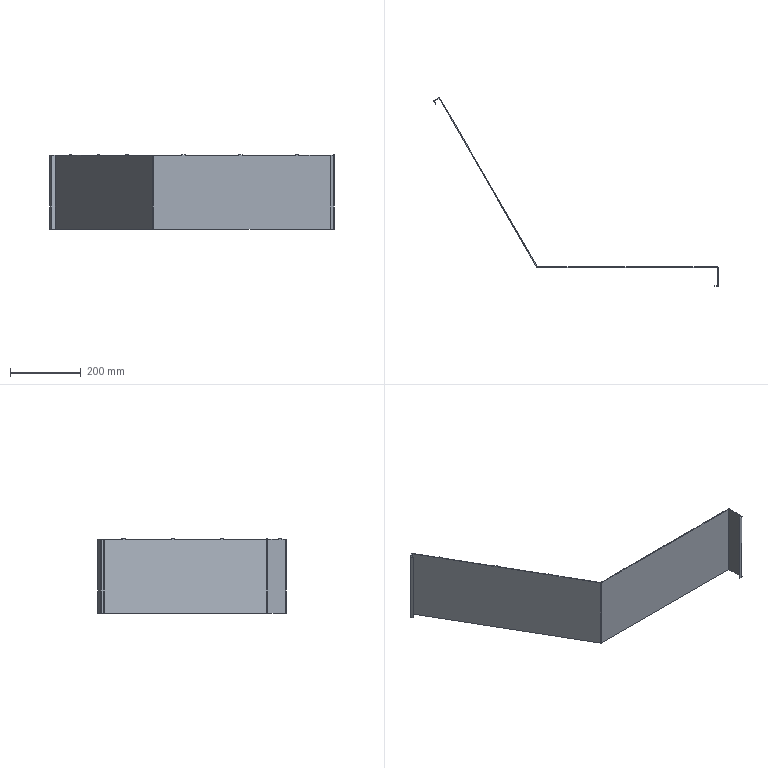Part | STEP file | zh004 | 1 solid | 56 faces | box 802.614 x 531.751 x 210 mm | volume 477513 mm3 | plane 44 | cylinder 12 | commonest cylinder face diameters 1 x6 5 x6